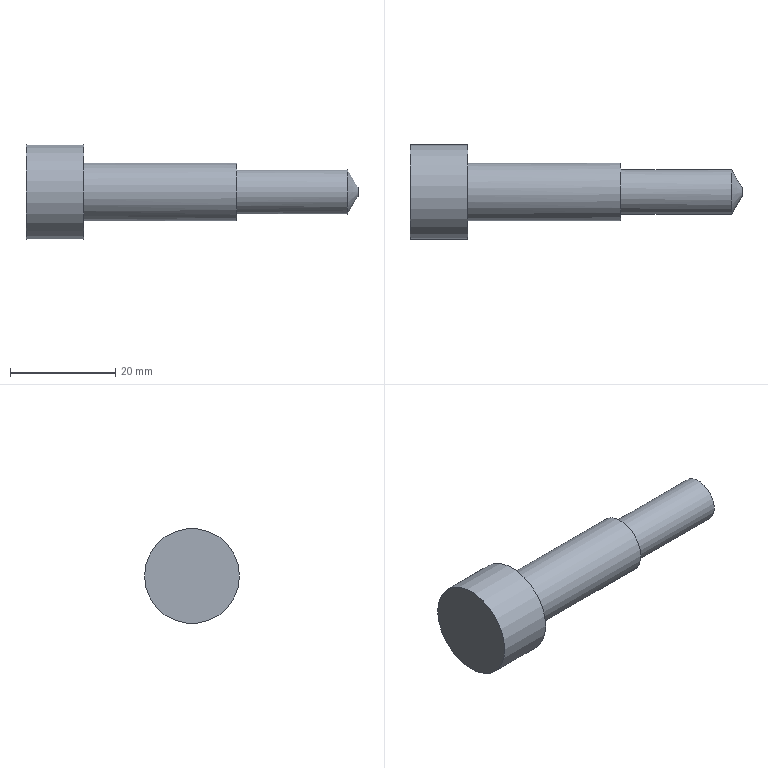Part | STEP file | solid 254 | 1 solid | 8 faces | box 63 x 18 x 18 mm | volume 6793 mm3 | plane 4 | cylinder 3 | cone 1 | commonest cylinder face diameters 8.5 x1 11 x1 18 x1